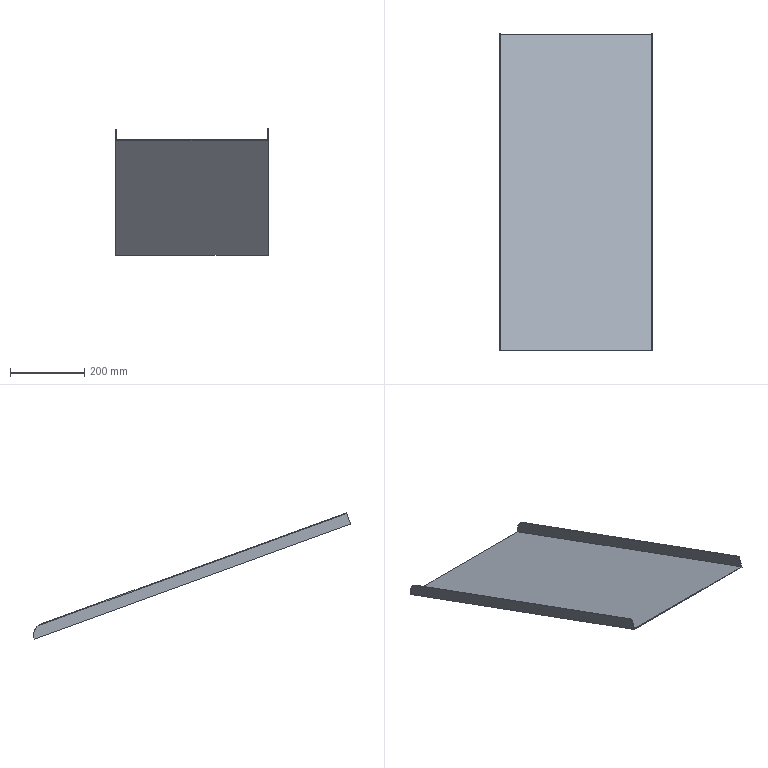Part | NX | features solid 2 | 1 solid | 12 faces | box 410 x 851.809 x 339.445 mm | volume 845547 mm3 | plane 10 | cylinder 2 | commonest cylinder face diameters 60 x2
STEP:
#1=CARTESIAN_POINT('',(-68.,1180.,-567.246));
#2=VERTEX_POINT('',#1);
#3=CARTESIAN_POINT('',(338.,1180.,-567.246));
#4=VERTEX_POINT('',#3);
#5=CARTESIAN_POINT('',(-625.,1180.,-567.246));
#6=DIRECTION('',(-1.,0.,0.));
#7=VECTOR('',#6,1000.);
#8=LINE('',#5,#7);
#9=EDGE_CURVE('',#2,#4,#8,.F.);
#10=ORIENTED_EDGE('',*,*,#9,.F.);
#11=CARTESIAN_POINT('',(-68.,330.684,-258.121));
#12=VERTEX_POINT('',#11);
#13=CARTESIAN_POINT('',(-68.,-154.316,-81.595));
#14=DIRECTION('',(0.,-0.9397,0.342));
#15=VECTOR('',#14,1000.);
#16=LINE('',#13,#15);
#17=EDGE_CURVE('',#2,#12,#16,.T.);
#18=ORIENTED_EDGE('',*,*,#17,.T.);
#19=CARTESIAN_POINT('',(338.,330.684,-258.121));
#20=VERTEX_POINT('',#19);
#21=CARTESIAN_POINT('',(-2928.754,330.684,-258.121));
#22=DIRECTION('',(1.,0.,0.));
#23=VECTOR('',#22,1000.);
#24=LINE('',#21,#23);
#25=EDGE_CURVE('',#12,#20,#24,.T.);
#26=ORIENTED_EDGE('',*,*,#25,.T.);
#27=CARTESIAN_POINT('',(338.,330.684,-258.121));
#28=DIRECTION('',(0.,0.9397,-0.342));
#29=VECTOR('',#28,1000.);
#30=LINE('',#27,#29);
#31=EDGE_CURVE('',#20,#4,#30,.T.);
#32=ORIENTED_EDGE('',*,*,#31,.T.);
#33=EDGE_LOOP('',(#10,#18,#26,#32));
#34=FACE_BOUND('',#33,.T.);
#35=CARTESIAN_POINT('',(-230.,-154.316,-81.595));
#36=DIRECTION('',(0.,0.342,0.9397));
#37=DIRECTION('',(1.,0.,0.));
#38=AXIS2_PLACEMENT_3D('',#35,#36,#37);
#39=PLANE('',#38);
#40=ADVANCED_FACE('',(#34),#39,.T.);
#41=CARTESIAN_POINT('',(-68.,1180.,-569.375));
#42=VERTEX_POINT('',#41);
#43=CARTESIAN_POINT('',(340.,1180.,-569.375));
#44=VERTEX_POINT('',#43);
#45=CARTESIAN_POINT('',(-625.,1180.,-569.375));
#46=DIRECTION('',(-1.,0.,0.));
#47=VECTOR('',#46,1000.);
#48=LINE('',#45,#47);
#49=EDGE_CURVE('',#42,#44,#48,.F.);
#50=ORIENTED_EDGE('',*,*,#49,.F.);
#51=CARTESIAN_POINT('',(-68.,1180.,-730.));
#52=DIRECTION('',(0.,0.,-1.));
#53=VECTOR('',#52,1000.);
#54=LINE('',#51,#53);
#55=EDGE_CURVE('',#42,#2,#54,.F.);
#56=ORIENTED_EDGE('',*,*,#55,.T.);
#57=ORIENTED_EDGE('',*,*,#9,.T.);
#58=CARTESIAN_POINT('',(340.,1180.,-567.246));
#59=VERTEX_POINT('',#58);
#60=CARTESIAN_POINT('',(340.,1180.,-567.246));
#61=DIRECTION('',(1.,0.,0.));
#62=VECTOR('',#61,1000.);
#63=LINE('',#60,#62);
#64=EDGE_CURVE('',#59,#4,#63,.F.);
#65=ORIENTED_EDGE('',*,*,#64,.F.);
#66=CARTESIAN_POINT('',(340.,1180.,-258.121));
#67=DIRECTION('',(0.,0.,1.));
#68=VECTOR('',#67,1000.);
#69=LINE('',#66,#68);
#70=EDGE_CURVE('',#59,#44,#69,.F.);
#71=ORIENTED_EDGE('',*,*,#70,.T.);
#72=EDGE_LOOP('',(#50,#56,#57,#65,#71));
#73=FACE_BOUND('',#72,.T.);
#74=CARTESIAN_POINT('',(-625.,1180.,-730.));
#75=DIRECTION('',(0.,-1.,0.));
#76=DIRECTION('',(1.,0.,0.));
#77=AXIS2_PLACEMENT_3D('',#74,#75,#76);
#78=PLANE('',#77);
#79=ADVANCED_FACE('',(#73),#78,.F.);
#80=CARTESIAN_POINT('',(340.,330.,-260.));
#81=VERTEX_POINT('',#80);
#82=CARTESIAN_POINT('',(340.,330.,-260.));
#83=DIRECTION('',(0.,0.9397,-0.342));
#84=VECTOR('',#83,1000.);
#85=LINE('',#82,#84);
#86=EDGE_CURVE('',#81,#44,#85,.T.);
#87=ORIENTED_EDGE('',*,*,#86,.T.);
#88=ORIENTED_EDGE('',*,*,#70,.F.);
#89=CARTESIAN_POINT('',(340.,1162.07,-528.795));
#90=VERTEX_POINT('',#89);
#91=CARTESIAN_POINT('',(340.,1151.809,-556.986));
#92=DIRECTION('',(1.,0.,0.));
#93=DIRECTION('',(0.,0.,-1.));
#94=AXIS2_PLACEMENT_3D('',#91,#92,#93);
#95=CIRCLE('',#94,30.);
#96=EDGE_CURVE('',#59,#90,#95,.T.);
#97=ORIENTED_EDGE('',*,*,#96,.T.);
#98=CARTESIAN_POINT('',(340.,340.945,-229.93));
#99=VERTEX_POINT('',#98);
#100=CARTESIAN_POINT('',(340.,340.945,-229.93));
#101=DIRECTION('',(0.,0.9397,-0.342));
#102=VECTOR('',#101,1000.);
#103=LINE('',#100,#102);
#104=EDGE_CURVE('',#99,#90,#103,.T.);
#105=ORIENTED_EDGE('',*,*,#104,.F.);
#106=CARTESIAN_POINT('',(340.,330.684,-258.121));
#107=DIRECTION('',(0.,-0.342,-0.9397));
#108=VECTOR('',#107,1000.);
#109=LINE('',#106,#108);
#110=EDGE_CURVE('',#99,#81,#109,.T.);
#111=ORIENTED_EDGE('',*,*,#110,.T.);
#112=EDGE_LOOP('',(#87,#88,#97,#105,#111));
#113=FACE_BOUND('',#112,.T.);
#114=CARTESIAN_POINT('',(340.,330.684,-258.121));
#115=DIRECTION('',(-1.,0.,0.));
#116=DIRECTION('',(0.,0.,1.));
#117=AXIS2_PLACEMENT_3D('',#114,#115,#116);
#118=PLANE('',#117);
#119=ADVANCED_FACE('',(#113),#118,.F.);
#120=CARTESIAN_POINT('',(-70.,340.261,-231.809));
#121=VERTEX_POINT('',#120);
#122=CARTESIAN_POINT('',(-70.,330.,-260.));
#123=VERTEX_POINT('',#122);
#124=CARTESIAN_POINT('',(-70.,330.684,-258.121));
#125=DIRECTION('',(0.,-0.342,-0.9397));
#126=VECTOR('',#125,1000.);
#127=LINE('',#124,#126);
#128=EDGE_CURVE('',#121,#123,#127,.T.);
#129=ORIENTED_EDGE('',*,*,#128,.F.);
#130=CARTESIAN_POINT('',(-70.,1162.07,-530.923));
#131=VERTEX_POINT('',#130);
#132=CARTESIAN_POINT('',(-70.,1190.261,-541.184));
#133=DIRECTION('',(0.,-0.9397,0.342));
#134=VECTOR('',#133,1000.);
#135=LINE('',#132,#134);
#136=EDGE_CURVE('',#131,#121,#135,.T.);
#137=ORIENTED_EDGE('',*,*,#136,.F.);
#138=CARTESIAN_POINT('',(-70.,1180.,-569.375));
#139=VERTEX_POINT('',#138);
#140=CARTESIAN_POINT('',(-70.,1151.809,-559.114));
#141=DIRECTION('',(-1.,0.,0.));
#142=DIRECTION('',(0.,0.,1.));
#143=AXIS2_PLACEMENT_3D('',#140,#141,#142);
#144=CIRCLE('',#143,30.);
#145=EDGE_CURVE('',#131,#139,#144,.T.);
#146=ORIENTED_EDGE('',*,*,#145,.T.);
#147=CARTESIAN_POINT('',(-70.,-155.,-83.474));
#148=DIRECTION('',(0.,-0.9397,0.342));
#149=VECTOR('',#148,1000.);
#150=LINE('',#147,#149);
#151=EDGE_CURVE('',#139,#123,#150,.T.);
#152=ORIENTED_EDGE('',*,*,#151,.T.);
#153=EDGE_LOOP('',(#129,#137,#146,#152));
#154=FACE_BOUND('',#153,.T.);
#155=CARTESIAN_POINT('',(-70.,-154.316,-81.595));
#156=DIRECTION('',(1.,0.,0.));
#157=DIRECTION('',(0.,0.,-1.));
#158=AXIS2_PLACEMENT_3D('',#155,#156,#157);
#159=PLANE('',#158);
#160=ADVANCED_FACE('',(#154),#159,.F.);
#161=CARTESIAN_POINT('',(-2928.754,330.,-260.));
#162=DIRECTION('',(1.,0.,0.));
#163=VECTOR('',#162,1000.);
#164=LINE('',#161,#163);
#165=EDGE_CURVE('',#123,#81,#164,.T.);
#166=ORIENTED_EDGE('',*,*,#165,.T.);
#167=ORIENTED_EDGE('',*,*,#110,.F.);
#168=CARTESIAN_POINT('',(338.,340.945,-229.93));
#169=VERTEX_POINT('',#168);
#170=CARTESIAN_POINT('',(340.,340.945,-229.93));
#171=DIRECTION('',(1.,0.,0.));
#172=VECTOR('',#171,1000.);
#173=LINE('',#170,#172);
#174=EDGE_CURVE('',#99,#169,#173,.F.);
#175=ORIENTED_EDGE('',*,*,#174,.T.);
#176=CARTESIAN_POINT('',(338.,330.684,-258.121));
#177=DIRECTION('',(0.,0.342,0.9397));
#178=VECTOR('',#177,1000.);
#179=LINE('',#176,#178);
#180=EDGE_CURVE('',#20,#169,#179,.T.);
#181=ORIENTED_EDGE('',*,*,#180,.F.);
#182=ORIENTED_EDGE('',*,*,#25,.F.);
#183=CARTESIAN_POINT('',(-68.,340.261,-231.809));
#184=VERTEX_POINT('',#183);
#185=CARTESIAN_POINT('',(-68.,330.,-260.));
#186=DIRECTION('',(0.,0.342,0.9397));
#187=VECTOR('',#186,1000.);
#188=LINE('',#185,#187);
#189=EDGE_CURVE('',#12,#184,#188,.T.);
#190=ORIENTED_EDGE('',*,*,#189,.T.);
#191=CARTESIAN_POINT('',(-70.,340.261,-231.809));
#192=DIRECTION('',(1.,0.,0.));
#193=VECTOR('',#192,1000.);
#194=LINE('',#191,#193);
#195=EDGE_CURVE('',#121,#184,#194,.T.);
#196=ORIENTED_EDGE('',*,*,#195,.F.);
#197=ORIENTED_EDGE('',*,*,#128,.T.);
#198=EDGE_LOOP('',(#166,#167,#175,#181,#182,#190,#196,#197));
#199=FACE_BOUND('',#198,.T.);
#200=CARTESIAN_POINT('',(-2928.754,330.684,-258.121));
#201=DIRECTION('',(0.,0.9397,-0.342));
#202=DIRECTION('',(0.,0.342,0.9397));
#203=AXIS2_PLACEMENT_3D('',#200,#201,#202);
#204=PLANE('',#203);
#205=ADVANCED_FACE('',(#199),#204,.F.);
#206=CARTESIAN_POINT('',(-625.,1180.,-569.375));
#207=DIRECTION('',(-1.,0.,0.));
#208=VECTOR('',#207,1000.);
#209=LINE('',#206,#208);
#210=EDGE_CURVE('',#139,#42,#209,.F.);
#211=ORIENTED_EDGE('',*,*,#210,.T.);
#212=ORIENTED_EDGE('',*,*,#49,.T.);
#213=ORIENTED_EDGE('',*,*,#86,.F.);
#214=ORIENTED_EDGE('',*,*,#165,.F.);
#215=ORIENTED_EDGE('',*,*,#151,.F.);
#216=EDGE_LOOP('',(#211,#212,#213,#214,#215));
#217=FACE_BOUND('',#216,.T.);
#218=CARTESIAN_POINT('',(-230.,-155.,-83.474));
#219=DIRECTION('',(0.,0.342,0.9397));
#220=DIRECTION('',(1.,0.,0.));
#221=AXIS2_PLACEMENT_3D('',#218,#219,#220);
#222=PLANE('',#221);
#223=ADVANCED_FACE('',(#217),#222,.F.);
#224=ORIENTED_EDGE('',*,*,#104,.T.);
#225=CARTESIAN_POINT('',(338.,1162.07,-528.795));
#226=VERTEX_POINT('',#225);
#227=CARTESIAN_POINT('',(340.,1162.07,-528.795));
#228=DIRECTION('',(1.,0.,0.));
#229=VECTOR('',#228,1000.);
#230=LINE('',#227,#229);
#231=EDGE_CURVE('',#90,#226,#230,.F.);
#232=ORIENTED_EDGE('',*,*,#231,.T.);
#233=CARTESIAN_POINT('',(338.,340.945,-229.93));
#234=DIRECTION('',(0.,0.9397,-0.342));
#235=VECTOR('',#234,1000.);
#236=LINE('',#233,#235);
#237=EDGE_CURVE('',#169,#226,#236,.T.);
#238=ORIENTED_EDGE('',*,*,#237,.F.);
#239=ORIENTED_EDGE('',*,*,#174,.F.);
#240=EDGE_LOOP('',(#224,#232,#238,#239));
#241=FACE_BOUND('',#240,.T.);
#242=CARTESIAN_POINT('',(340.,340.945,-229.93));
#243=DIRECTION('',(0.,-0.342,-0.9397));
#244=DIRECTION('',(0.,0.9397,-0.342));
#245=AXIS2_PLACEMENT_3D('',#242,#243,#244);
#246=PLANE('',#245);
#247=ADVANCED_FACE('',(#241),#246,.F.);
#248=ORIENTED_EDGE('',*,*,#237,.T.);
#249=CARTESIAN_POINT('',(338.,1151.809,-556.986));
#250=DIRECTION('',(1.,0.,0.));
#251=DIRECTION('',(0.,0.,-1.));
#252=AXIS2_PLACEMENT_3D('',#249,#250,#251);
#253=CIRCLE('',#252,30.);
#254=EDGE_CURVE('',#226,#4,#253,.F.);
#255=ORIENTED_EDGE('',*,*,#254,.T.);
#256=ORIENTED_EDGE('',*,*,#31,.F.);
#257=ORIENTED_EDGE('',*,*,#180,.T.);
#258=EDGE_LOOP('',(#248,#255,#256,#257));
#259=FACE_BOUND('',#258,.T.);
#260=CARTESIAN_POINT('',(338.,330.684,-258.121));
#261=DIRECTION('',(1.,0.,0.));
#262=DIRECTION('',(0.,0.,-1.));
#263=AXIS2_PLACEMENT_3D('',#260,#261,#262);
#264=PLANE('',#263);
#265=ADVANCED_FACE('',(#259),#264,.F.);
#266=ORIENTED_EDGE('',*,*,#96,.F.);
#267=ORIENTED_EDGE('',*,*,#64,.T.);
#268=ORIENTED_EDGE('',*,*,#254,.F.);
#269=ORIENTED_EDGE('',*,*,#231,.F.);
#270=EDGE_LOOP('',(#266,#267,#268,#269));
#271=FACE_BOUND('',#270,.T.);
#272=CARTESIAN_POINT('',(340.,1151.809,-556.986));
#273=DIRECTION('',(1.,0.,0.));
#274=DIRECTION('',(0.,0.,-1.));
#275=AXIS2_PLACEMENT_3D('',#272,#273,#274);
#276=CYLINDRICAL_SURFACE('',#275,30.);
#277=ADVANCED_FACE('',(#271),#276,.T.);
#278=CARTESIAN_POINT('',(-68.,1162.07,-530.923));
#279=VERTEX_POINT('',#278);
#280=CARTESIAN_POINT('',(-68.,1190.261,-541.184));
#281=DIRECTION('',(0.,-0.9397,0.342));
#282=VECTOR('',#281,1000.);
#283=LINE('',#280,#282);
#284=EDGE_CURVE('',#279,#184,#283,.T.);
#285=ORIENTED_EDGE('',*,*,#284,.F.);
#286=CARTESIAN_POINT('',(-70.,1162.07,-530.923));
#287=DIRECTION('',(-1.,0.,0.));
#288=VECTOR('',#287,1000.);
#289=LINE('',#286,#288);
#290=EDGE_CURVE('',#279,#131,#289,.T.);
#291=ORIENTED_EDGE('',*,*,#290,.T.);
#292=ORIENTED_EDGE('',*,*,#136,.T.);
#293=ORIENTED_EDGE('',*,*,#195,.T.);
#294=EDGE_LOOP('',(#285,#291,#292,#293));
#295=FACE_BOUND('',#294,.T.);
#296=CARTESIAN_POINT('',(-70.,1190.261,-541.184));
#297=DIRECTION('',(0.,-0.342,-0.9397));
#298=DIRECTION('',(0.,-0.9397,0.342));
#299=AXIS2_PLACEMENT_3D('',#296,#297,#298);
#300=PLANE('',#299);
#301=ADVANCED_FACE('',(#295),#300,.F.);
#302=ORIENTED_EDGE('',*,*,#17,.F.);
#303=ORIENTED_EDGE('',*,*,#55,.F.);
#304=CARTESIAN_POINT('',(-68.,1151.809,-559.114));
#305=DIRECTION('',(-1.,0.,0.));
#306=DIRECTION('',(0.,0.,1.));
#307=AXIS2_PLACEMENT_3D('',#304,#305,#306);
#308=CIRCLE('',#307,30.);
#309=EDGE_CURVE('',#42,#279,#308,.F.);
#310=ORIENTED_EDGE('',*,*,#309,.T.);
#311=ORIENTED_EDGE('',*,*,#284,.T.);
#312=ORIENTED_EDGE('',*,*,#189,.F.);
#313=EDGE_LOOP('',(#302,#303,#310,#311,#312));
#314=FACE_BOUND('',#313,.T.);
#315=CARTESIAN_POINT('',(-68.,1180.,-569.375));
#316=DIRECTION('',(-1.,0.,0.));
#317=DIRECTION('',(0.,0.,1.));
#318=AXIS2_PLACEMENT_3D('',#315,#316,#317);
#319=PLANE('',#318);
#320=ADVANCED_FACE('',(#314),#319,.F.);
#321=ORIENTED_EDGE('',*,*,#145,.F.);
#322=ORIENTED_EDGE('',*,*,#290,.F.);
#323=ORIENTED_EDGE('',*,*,#309,.F.);
#324=ORIENTED_EDGE('',*,*,#210,.F.);
#325=EDGE_LOOP('',(#321,#322,#323,#324));
#326=FACE_BOUND('',#325,.T.);
#327=CARTESIAN_POINT('',(-70.,1151.809,-559.114));
#328=DIRECTION('',(1.,0.,0.));
#329=DIRECTION('',(0.,0.,-1.));
#330=AXIS2_PLACEMENT_3D('',#327,#328,#329);
#331=CYLINDRICAL_SURFACE('',#330,30.);
#332=ADVANCED_FACE('',(#326),#331,.T.);
#333=CLOSED_SHELL('',(#40,#79,#119,#160,#205,#223,#247,#265,#277,#301,#320,#332));
#334=MANIFOLD_SOLID_BREP('',#333);
#335=(LENGTH_UNIT()NAMED_UNIT(*)SI_UNIT(.MILLI.,.METRE.));
#336=UNCERTAINTY_MEASURE_WITH_UNIT(LENGTH_MEASURE(0.00001),#335,'','');
#337=(NAMED_UNIT(*)PLANE_ANGLE_UNIT()SI_UNIT($,.RADIAN.));
#338=(NAMED_UNIT(*)SI_UNIT($,.STERADIAN.)SOLID_ANGLE_UNIT());
#339=(GEOMETRIC_REPRESENTATION_CONTEXT(3)GLOBAL_UNCERTAINTY_ASSIGNED_CONTEXT((#336))GLOBAL_UNIT_ASSIGNED_CONTEXT((#335,#337,#338))REPRESENTATION_CONTEXT('',''));
#340=ADVANCED_BREP_SHAPE_REPRESENTATION('',(#334),#339);